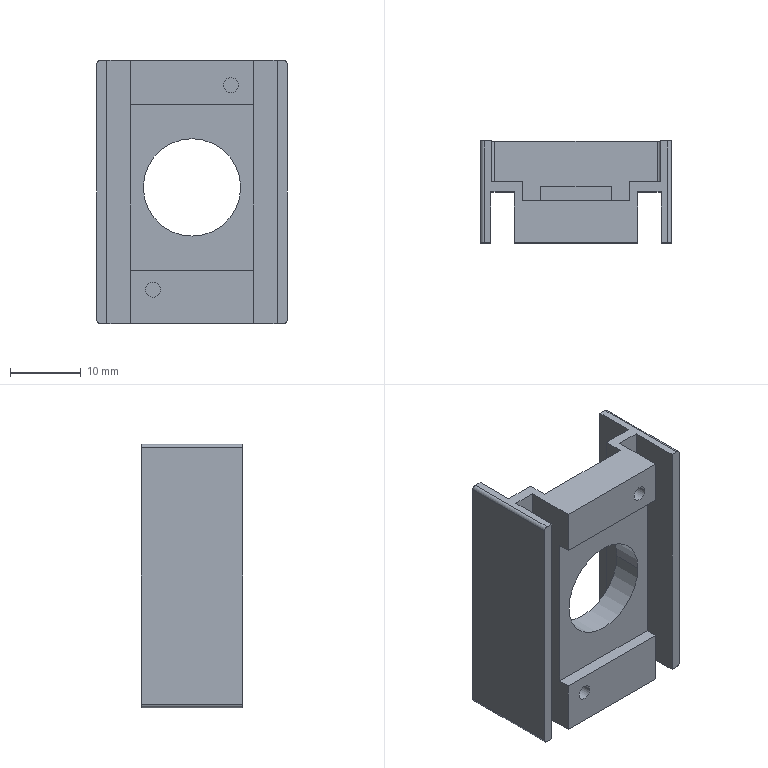Part | STEP file | _X2_751F4E45_X0_MS731-1_X2_8_15 | 1 solid | 53 faces | box 27 x 14.4 x 37.3 mm | volume 4925 mm3 | plane 35 | cylinder 14 | cone 4 | commonest cylinder face diameters 1 x6 2.1 x4 5 x2 13.8 x2